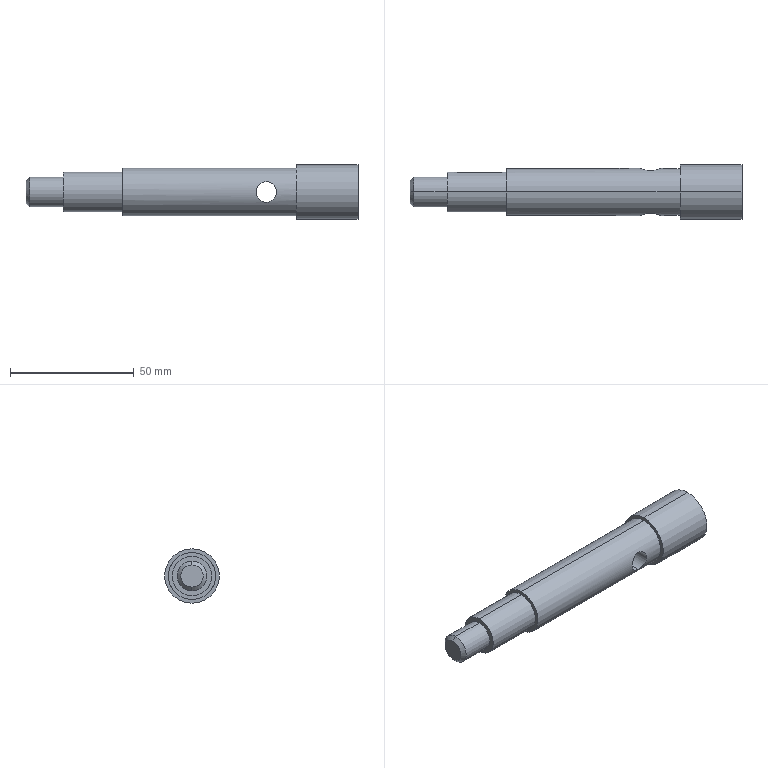Part | SolidWorks | features Cut 2, Chamfer 1, RevCut 1, Revolution 1 | 1 solid | 25 faces | box 134 x 22 x 22 mm | volume 34206 mm3 | cylinder 15 | plane 8 | cone 2 | commonest cylinder face diameters 2.8 x4 8.3 x2 12 x2 16 x2 19 x2 22 x2
STEP:
#1=CARTESIAN_POINT('',(-52.374,0.,4.5));
#2=VERTEX_POINT('',#1);
#3=CARTESIAN_POINT('',(-52.374,0.,-4.5));
#4=VERTEX_POINT('',#3);
#5=CARTESIAN_POINT('',(-52.374,0.,0.));
#6=DIRECTION('',(-1.,0.,0.));
#7=DIRECTION('',(0.,0.,-1.));
#8=AXIS2_PLACEMENT_3D('',#5,#6,#7);
#9=CIRCLE('',#8,4.5);
#10=EDGE_CURVE('',#2,#4,#9,.T.);
#11=ORIENTED_EDGE('',*,*,#10,.F.);
#12=CARTESIAN_POINT('',(-50.874,0.,6.));
#13=VERTEX_POINT('',#12);
#14=CARTESIAN_POINT('',(-52.374,0.,4.5));
#15=DIRECTION('',(0.7071,0.,0.7071));
#16=VECTOR('',#15,1000.);
#17=LINE('',#14,#16);
#18=EDGE_CURVE('',#2,#13,#17,.T.);
#19=ORIENTED_EDGE('',*,*,#18,.T.);
#20=CARTESIAN_POINT('',(-50.874,0.,-6.));
#21=VERTEX_POINT('',#20);
#22=CARTESIAN_POINT('',(-50.874,0.,0.));
#23=DIRECTION('',(1.,0.,0.));
#24=DIRECTION('',(0.,0.,-1.));
#25=AXIS2_PLACEMENT_3D('',#22,#23,#24);
#26=CIRCLE('',#25,6.);
#27=EDGE_CURVE('',#21,#13,#26,.T.);
#28=ORIENTED_EDGE('',*,*,#27,.F.);
#29=CARTESIAN_POINT('',(-52.374,0.,-4.5));
#30=DIRECTION('',(0.7071,0.,-0.7071));
#31=VECTOR('',#30,1000.);
#32=LINE('',#29,#31);
#33=EDGE_CURVE('',#4,#21,#32,.T.);
#34=ORIENTED_EDGE('',*,*,#33,.F.);
#35=EDGE_LOOP('',(#11,#19,#28,#34));
#36=FACE_OUTER_BOUND('',#35,.T.);
#37=CARTESIAN_POINT('',(-52.374,0.,0.));
#38=DIRECTION('',(1.,0.,0.));
#39=DIRECTION('',(0.,0.,-1.));
#40=AXIS2_PLACEMENT_3D('',#37,#38,#39);
#41=CONICAL_SURFACE('',#40,4.5,0.7854);
#42=ADVANCED_FACE('',(#36),#41,.T.);
#43=CARTESIAN_POINT('',(37.626,0.,1.4));
#44=VERTEX_POINT('',#43);
#45=CARTESIAN_POINT('',(37.626,0.,-1.4));
#46=VERTEX_POINT('',#45);
#47=CARTESIAN_POINT('',(37.626,0.,0.));
#48=DIRECTION('',(1.,0.,0.));
#49=DIRECTION('',(0.,0.,-1.));
#50=AXIS2_PLACEMENT_3D('',#47,#48,#49);
#51=CIRCLE('',#50,1.4);
#52=EDGE_CURVE('',#44,#46,#51,.T.);
#53=ORIENTED_EDGE('',*,*,#52,.F.);
#54=CARTESIAN_POINT('',(40.72,0.,1.4));
#55=VERTEX_POINT('',#54);
#56=CARTESIAN_POINT('',(37.626,0.,1.4));
#57=DIRECTION('',(1.,0.,0.));
#58=VECTOR('',#57,1000.);
#59=LINE('',#56,#58);
#60=EDGE_CURVE('',#44,#55,#59,.T.);
#61=ORIENTED_EDGE('',*,*,#60,.T.);
#62=CARTESIAN_POINT('',(40.72,0.,-1.4));
#63=VERTEX_POINT('',#62);
#64=CARTESIAN_POINT('',(40.72,0.,1.4));
#65=CARTESIAN_POINT('',(40.72,-0.1836,1.4));
#66=CARTESIAN_POINT('',(40.706,-0.369,1.363));
#67=CARTESIAN_POINT('',(40.671,-0.6223,1.257));
#68=CARTESIAN_POINT('',(40.657,-0.7041,1.213));
#69=CARTESIAN_POINT('',(40.628,-0.8552,1.112));
#70=CARTESIAN_POINT('',(40.612,-0.9252,1.055));
#71=CARTESIAN_POINT('',(40.564,-1.119,0.8607));
#72=CARTESIAN_POINT('',(40.534,-1.222,0.708));
#73=CARTESIAN_POINT('',(40.5,-1.328,0.4527));
#74=CARTESIAN_POINT('',(40.491,-1.355,0.3652));
#75=CARTESIAN_POINT('',(40.48,-1.391,0.1854));
#76=CARTESIAN_POINT('',(40.476,-1.4,0.092));
#77=CARTESIAN_POINT('',(40.476,-1.4,-0.1847));
#78=CARTESIAN_POINT('',(40.489,-1.363,-0.3697));
#79=CARTESIAN_POINT('',(40.533,-1.222,-0.7069));
#80=CARTESIAN_POINT('',(40.565,-1.118,-0.8618));
#81=CARTESIAN_POINT('',(40.612,-0.9256,-1.054));
#82=CARTESIAN_POINT('',(40.628,-0.8542,-1.113));
#83=CARTESIAN_POINT('',(40.658,-0.703,-1.214));
#84=CARTESIAN_POINT('',(40.671,-0.623,-1.257));
#85=CARTESIAN_POINT('',(40.694,-0.4537,-1.328));
#86=CARTESIAN_POINT('',(40.704,-0.3645,-1.355));
#87=CARTESIAN_POINT('',(40.716,-0.1848,-1.391));
#88=CARTESIAN_POINT('',(40.72,-0.09322,-1.4));
#89=CARTESIAN_POINT('',(40.72,0.,-1.4));
#90=B_SPLINE_CURVE_WITH_KNOTS('',3,(#64,#65,#66,#67,#68,#69,#70,#71,#72,#73,#74,#75,#76,#77,#78,#79,#80,#81,#82,#83,#84,#85,#86,#87,#88,#89),.UNSPECIFIED.,.F.,.F.,(4,2,2,2,2,2,2,2,2,2,2,2,4),(0.00441,0.004961,0.005236,0.005512,0.006063,0.006338,0.006614,0.007165,0.007716,0.007991,0.008267,0.008542,0.008818),.UNSPECIFIED.);
#91=EDGE_CURVE('',#55,#63,#90,.T.);
#92=ORIENTED_EDGE('',*,*,#91,.T.);
#93=CARTESIAN_POINT('',(37.626,0.,-1.4));
#94=DIRECTION('',(1.,0.,0.));
#95=VECTOR('',#94,1000.);
#96=LINE('',#93,#95);
#97=EDGE_CURVE('',#46,#63,#96,.T.);
#98=ORIENTED_EDGE('',*,*,#97,.F.);
#99=EDGE_LOOP('',(#53,#61,#92,#98));
#100=FACE_OUTER_BOUND('',#99,.T.);
#101=CARTESIAN_POINT('',(37.626,0.,0.));
#102=DIRECTION('',(1.,0.,0.));
#103=DIRECTION('',(0.,0.,-1.));
#104=AXIS2_PLACEMENT_3D('',#101,#102,#103);
#105=CYLINDRICAL_SURFACE('',#104,1.4);
#106=ADVANCED_FACE('',(#100),#105,.F.);
#107=CARTESIAN_POINT('',(40.72,0.,-1.4));
#108=CARTESIAN_POINT('',(40.72,0.09325,-1.4));
#109=CARTESIAN_POINT('',(40.716,0.1848,-1.391));
#110=CARTESIAN_POINT('',(40.704,0.3646,-1.355));
#111=CARTESIAN_POINT('',(40.694,0.4539,-1.328));
#112=CARTESIAN_POINT('',(40.66,0.7077,-1.222));
#113=CARTESIAN_POINT('',(40.628,0.862,-1.118));
#114=CARTESIAN_POINT('',(40.565,1.118,-0.8616));
#115=CARTESIAN_POINT('',(40.533,1.222,-0.7065));
#116=CARTESIAN_POINT('',(40.489,1.362,-0.37));
#117=CARTESIAN_POINT('',(40.476,1.4,-0.1849));
#118=CARTESIAN_POINT('',(40.476,1.4,0.09146));
#119=CARTESIAN_POINT('',(40.479,1.391,0.185));
#120=CARTESIAN_POINT('',(40.491,1.355,0.3652));
#121=CARTESIAN_POINT('',(40.5,1.328,0.4528));
#122=CARTESIAN_POINT('',(40.534,1.222,0.7085));
#123=CARTESIAN_POINT('',(40.565,1.118,0.8619));
#124=CARTESIAN_POINT('',(40.612,0.9248,1.055));
#125=CARTESIAN_POINT('',(40.628,0.8548,1.112));
#126=CARTESIAN_POINT('',(40.657,0.7036,1.214));
#127=CARTESIAN_POINT('',(40.671,0.6218,1.258));
#128=CARTESIAN_POINT('',(40.706,0.369,1.363));
#129=CARTESIAN_POINT('',(40.72,0.1837,1.4));
#130=CARTESIAN_POINT('',(40.72,0.,1.4));
#131=B_SPLINE_CURVE_WITH_KNOTS('',3,(#107,#108,#109,#110,#111,#112,#113,#114,#115,#116,#117,#118,#119,#120,#121,#122,#123,#124,#125,#126,#127,#128,#129,#130),.UNSPECIFIED.,.F.,.F.,(4,2,2,2,2,2,2,2,2,2,2,4),(0.,0.0002756,0.0005512,0.001102,0.001654,0.002205,0.00248,0.002756,0.003307,0.003583,0.003858,0.00441),.UNSPECIFIED.);
#132=EDGE_CURVE('',#63,#55,#131,.T.);
#133=ORIENTED_EDGE('',*,*,#132,.F.);
#134=ORIENTED_EDGE('',*,*,#91,.F.);
#135=EDGE_LOOP('',(#133,#134));
#136=FACE_BOUND('',#135,.T.);
#137=CARTESIAN_POINT('',(44.626,-8.546,-4.15));
#138=VERTEX_POINT('',#137);
#139=CARTESIAN_POINT('',(44.626,-8.546,4.15));
#140=VERTEX_POINT('',#139);
#141=CARTESIAN_POINT('',(44.626,-8.546,-4.15));
#142=CARTESIAN_POINT('',(44.353,-8.546,-4.15));
#143=CARTESIAN_POINT('',(44.075,-8.559,-4.122));
#144=CARTESIAN_POINT('',(43.538,-8.611,-4.014));
#145=CARTESIAN_POINT('',(43.278,-8.648,-3.934));
#146=CARTESIAN_POINT('',(42.776,-8.74,-3.724));
#147=CARTESIAN_POINT('',(42.536,-8.795,-3.595));
#148=CARTESIAN_POINT('',(42.091,-8.911,-3.296));
#149=CARTESIAN_POINT('',(41.881,-8.974,-3.124));
#150=CARTESIAN_POINT('',(41.501,-9.097,-2.744));
#151=CARTESIAN_POINT('',(41.331,-9.158,-2.537));
#152=CARTESIAN_POINT('',(41.032,-9.27,-2.092));
#153=CARTESIAN_POINT('',(40.901,-9.322,-1.849));
#154=CARTESIAN_POINT('',(40.693,-9.407,-1.349));
#155=CARTESIAN_POINT('',(40.613,-9.441,-1.09));
#156=CARTESIAN_POINT('',(40.504,-9.488,-0.5531));
#157=CARTESIAN_POINT('',(40.476,-9.5,-0.275));
#158=CARTESIAN_POINT('',(40.476,-9.5,0.2725));
#159=CARTESIAN_POINT('',(40.503,-9.488,0.5464));
#160=CARTESIAN_POINT('',(40.612,-9.441,1.088));
#161=CARTESIAN_POINT('',(40.692,-9.407,1.349));
#162=CARTESIAN_POINT('',(40.901,-9.322,1.849));
#163=CARTESIAN_POINT('',(41.032,-9.27,2.092));
#164=CARTESIAN_POINT('',(41.332,-9.158,2.538));
#165=CARTESIAN_POINT('',(41.502,-9.097,2.745));
#166=CARTESIAN_POINT('',(42.074,-8.911,3.316));
#167=CARTESIAN_POINT('',(42.523,-8.787,3.619));
#168=CARTESIAN_POINT('',(43.278,-8.648,3.934));
#169=CARTESIAN_POINT('',(43.538,-8.611,4.014));
#170=CARTESIAN_POINT('',(44.071,-8.56,4.122));
#171=CARTESIAN_POINT('',(44.349,-8.546,4.15));
#172=CARTESIAN_POINT('',(44.626,-8.546,4.15));
#173=B_SPLINE_CURVE_WITH_KNOTS('',3,(#141,#142,#143,#144,#145,#146,#147,#148,#149,#150,#151,#152,#153,#154,#155,#156,#157,#158,#159,#160,#161,#162,#163,#164,#165,#166,#167,#168,#169,#170,#171,#172),.UNSPECIFIED.,.F.,.F.,(4,2,2,2,2,2,2,2,2,2,2,2,2,2,2,4),(0.01314,0.01396,0.01478,0.0156,0.01642,0.01724,0.01806,0.01889,0.01971,0.02053,0.02135,0.02217,0.02299,0.02463,0.02545,0.02627),.UNSPECIFIED.);
#174=EDGE_CURVE('',#138,#140,#173,.T.);
#175=ORIENTED_EDGE('',*,*,#174,.F.);
#176=CARTESIAN_POINT('',(44.626,8.546,-4.15));
#177=VERTEX_POINT('',#176);
#178=CARTESIAN_POINT('',(44.626,-11.,-4.15));
#179=DIRECTION('',(0.,1.,0.));
#180=VECTOR('',#179,1000.);
#181=LINE('',#178,#180);
#182=EDGE_CURVE('',#138,#177,#181,.T.);
#183=ORIENTED_EDGE('',*,*,#182,.T.);
#184=CARTESIAN_POINT('',(44.626,8.546,4.15));
#185=VERTEX_POINT('',#184);
#186=CARTESIAN_POINT('',(44.626,8.546,4.15));
#187=CARTESIAN_POINT('',(44.348,8.546,4.15));
#188=CARTESIAN_POINT('',(44.076,8.559,4.122));
#189=CARTESIAN_POINT('',(43.541,8.61,4.015));
#190=CARTESIAN_POINT('',(43.276,8.648,3.933));
#191=CARTESIAN_POINT('',(42.775,8.74,3.724));
#192=CARTESIAN_POINT('',(42.538,8.794,3.597));
#193=CARTESIAN_POINT('',(42.09,8.911,3.296));
#194=CARTESIAN_POINT('',(41.881,8.974,3.124));
#195=CARTESIAN_POINT('',(41.503,9.097,2.746));
#196=CARTESIAN_POINT('',(41.331,9.158,2.538));
#197=CARTESIAN_POINT('',(41.029,9.271,2.088));
#198=CARTESIAN_POINT('',(40.902,9.321,1.851));
#199=CARTESIAN_POINT('',(40.693,9.407,1.352));
#200=CARTESIAN_POINT('',(40.612,9.441,1.087));
#201=CARTESIAN_POINT('',(40.504,9.488,0.5491));
#202=CARTESIAN_POINT('',(40.477,9.5,0.2772));
#203=CARTESIAN_POINT('',(40.476,9.5,-0.2726));
#204=CARTESIAN_POINT('',(40.504,9.488,-0.5512));
#205=CARTESIAN_POINT('',(40.612,9.441,-1.087));
#206=CARTESIAN_POINT('',(40.692,9.407,-1.349));
#207=CARTESIAN_POINT('',(40.904,9.321,-1.854));
#208=CARTESIAN_POINT('',(41.032,9.27,-2.092));
#209=CARTESIAN_POINT('',(41.332,9.158,-2.538));
#210=CARTESIAN_POINT('',(41.506,9.096,-2.749));
#211=CARTESIAN_POINT('',(41.885,8.973,-3.127));
#212=CARTESIAN_POINT('',(42.091,8.911,-3.297));
#213=CARTESIAN_POINT('',(42.539,8.794,-3.597));
#214=CARTESIAN_POINT('',(42.78,8.739,-3.726));
#215=CARTESIAN_POINT('',(43.278,8.648,-3.934));
#216=CARTESIAN_POINT('',(43.537,8.611,-4.014));
#217=CARTESIAN_POINT('',(44.08,8.559,-4.123));
#218=CARTESIAN_POINT('',(44.353,8.546,-4.15));
#219=CARTESIAN_POINT('',(44.626,8.546,-4.15));
#220=B_SPLINE_CURVE_WITH_KNOTS('',3,(#186,#187,#188,#189,#190,#191,#192,#193,#194,#195,#196,#197,#198,#199,#200,#201,#202,#203,#204,#205,#206,#207,#208,#209,#210,#211,#212,#213,#214,#215,#216,#217,#218,#219),.UNSPECIFIED.,.F.,.F.,(4,2,2,2,2,2,2,2,2,2,2,2,2,2,2,2,4),(0.,0.0008214,0.001643,0.002464,0.003285,0.004107,0.004928,0.00575,0.006571,0.007392,0.008214,0.009035,0.009856,0.01068,0.0115,0.01232,0.01314),.UNSPECIFIED.);
#221=EDGE_CURVE('',#185,#177,#220,.T.);
#222=ORIENTED_EDGE('',*,*,#221,.F.);
#223=CARTESIAN_POINT('',(44.626,-11.,4.15));
#224=DIRECTION('',(0.,1.,0.));
#225=VECTOR('',#224,1000.);
#226=LINE('',#223,#225);
#227=EDGE_CURVE('',#140,#185,#226,.T.);
#228=ORIENTED_EDGE('',*,*,#227,.F.);
#229=EDGE_LOOP('',(#175,#183,#222,#228));
#230=FACE_OUTER_BOUND('',#229,.T.);
#231=CARTESIAN_POINT('',(44.626,-11.,0.));
#232=DIRECTION('',(0.,1.,0.));
#233=DIRECTION('',(0.,0.,1.));
#234=AXIS2_PLACEMENT_3D('',#231,#232,#233);
#235=CYLINDRICAL_SURFACE('',#234,4.15);
#236=ADVANCED_FACE('',(#136,#230),#235,.F.);
#237=CARTESIAN_POINT('',(48.533,0.,-1.4));
#238=VERTEX_POINT('',#237);
#239=CARTESIAN_POINT('',(48.533,0.,1.4));
#240=VERTEX_POINT('',#239);
#241=CARTESIAN_POINT('',(48.533,0.,-1.4));
#242=CARTESIAN_POINT('',(48.533,-0.09325,-1.4));
#243=CARTESIAN_POINT('',(48.536,-0.1848,-1.391));
#244=CARTESIAN_POINT('',(48.549,-0.3646,-1.355));
#245=CARTESIAN_POINT('',(48.558,-0.4539,-1.328));
#246=CARTESIAN_POINT('',(48.593,-0.7077,-1.222));
#247=CARTESIAN_POINT('',(48.625,-0.862,-1.118));
#248=CARTESIAN_POINT('',(48.688,-1.118,-0.8616));
#249=CARTESIAN_POINT('',(48.719,-1.222,-0.7065));
#250=CARTESIAN_POINT('',(48.763,-1.362,-0.37));
#251=CARTESIAN_POINT('',(48.776,-1.4,-0.1849));
#252=CARTESIAN_POINT('',(48.776,-1.4,0.09146));
#253=CARTESIAN_POINT('',(48.773,-1.391,0.185));
#254=CARTESIAN_POINT('',(48.761,-1.355,0.3652));
#255=CARTESIAN_POINT('',(48.752,-1.328,0.4528));
#256=CARTESIAN_POINT('',(48.719,-1.222,0.7085));
#257=CARTESIAN_POINT('',(48.688,-1.118,0.8619));
#258=CARTESIAN_POINT('',(48.641,-0.9248,1.055));
#259=CARTESIAN_POINT('',(48.625,-0.8548,1.112));
#260=CARTESIAN_POINT('',(48.595,-0.7036,1.214));
#261=CARTESIAN_POINT('',(48.581,-0.6218,1.258));
#262=CARTESIAN_POINT('',(48.547,-0.369,1.363));
#263=CARTESIAN_POINT('',(48.533,-0.1837,1.4));
#264=CARTESIAN_POINT('',(48.533,0.,1.4));
#265=B_SPLINE_CURVE_WITH_KNOTS('',3,(#241,#242,#243,#244,#245,#246,#247,#248,#249,#250,#251,#252,#253,#254,#255,#256,#257,#258,#259,#260,#261,#262,#263,#264),.UNSPECIFIED.,.F.,.F.,(4,2,2,2,2,2,2,2,2,2,2,4),(0.,0.0002756,0.0005512,0.001102,0.001654,0.002205,0.00248,0.002756,0.003307,0.003583,0.003858,0.00441),.UNSPECIFIED.);
#266=EDGE_CURVE('',#238,#240,#265,.T.);
#267=ORIENTED_EDGE('',*,*,#266,.T.);
#268=CARTESIAN_POINT('',(81.626,0.,1.4));
#269=VERTEX_POINT('',#268);
#270=CARTESIAN_POINT('',(37.626,0.,1.4));
#271=DIRECTION('',(1.,0.,0.));
#272=VECTOR('',#271,1000.);
#273=LINE('',#270,#272);
#274=EDGE_CURVE('',#240,#269,#273,.T.);
#275=ORIENTED_EDGE('',*,*,#274,.T.);
#276=CARTESIAN_POINT('',(81.626,0.,-1.4));
#277=VERTEX_POINT('',#276);
#278=CARTESIAN_POINT('',(81.626,0.,0.));
#279=DIRECTION('',(1.,0.,0.));
#280=DIRECTION('',(0.,0.,-1.));
#281=AXIS2_PLACEMENT_3D('',#278,#279,#280);
#282=CIRCLE('',#281,1.4);
#283=EDGE_CURVE('',#269,#277,#282,.T.);
#284=ORIENTED_EDGE('',*,*,#283,.T.);
#285=CARTESIAN_POINT('',(37.626,0.,-1.4));
#286=DIRECTION('',(1.,0.,0.));
#287=VECTOR('',#286,1000.);
#288=LINE('',#285,#287);
#289=EDGE_CURVE('',#238,#277,#288,.T.);
#290=ORIENTED_EDGE('',*,*,#289,.F.);
#291=EDGE_LOOP('',(#267,#275,#284,#290));
#292=FACE_OUTER_BOUND('',#291,.T.);
#293=CARTESIAN_POINT('',(37.626,0.,0.));
#294=DIRECTION('',(1.,0.,0.));
#295=DIRECTION('',(0.,0.,-1.));
#296=AXIS2_PLACEMENT_3D('',#293,#294,#295);
#297=CYLINDRICAL_SURFACE('',#296,1.4);
#298=ADVANCED_FACE('',(#292),#297,.F.);
#299=CARTESIAN_POINT('',(-37.374,0.,6.));
#300=VERTEX_POINT('',#299);
#301=CARTESIAN_POINT('',(-37.374,0.,-6.));
#302=VERTEX_POINT('',#301);
#303=CARTESIAN_POINT('',(-37.374,0.,0.));
#304=DIRECTION('',(-1.,0.,0.));
#305=DIRECTION('',(0.,0.,1.));
#306=AXIS2_PLACEMENT_3D('',#303,#304,#305);
#307=CIRCLE('',#306,6.);
#308=EDGE_CURVE('',#300,#302,#307,.T.);
#309=ORIENTED_EDGE('',*,*,#308,.T.);
#310=CARTESIAN_POINT('',(-52.374,0.,-6.));
#311=DIRECTION('',(-1.,0.,0.));
#312=VECTOR('',#311,1000.);
#313=LINE('',#310,#312);
#314=EDGE_CURVE('',#302,#21,#313,.T.);
#315=ORIENTED_EDGE('',*,*,#314,.T.);
#316=ORIENTED_EDGE('',*,*,#27,.T.);
#317=CARTESIAN_POINT('',(-52.374,0.,6.));
#318=DIRECTION('',(-1.,0.,0.));
#319=VECTOR('',#318,1000.);
#320=LINE('',#317,#319);
#321=EDGE_CURVE('',#300,#13,#320,.T.);
#322=ORIENTED_EDGE('',*,*,#321,.F.);
#323=EDGE_LOOP('',(#309,#315,#316,#322));
#324=FACE_OUTER_BOUND('',#323,.T.);
#325=CARTESIAN_POINT('',(-52.374,0.,0.));
#326=DIRECTION('',(-1.,0.,0.));
#327=DIRECTION('',(0.,0.,1.));
#328=AXIS2_PLACEMENT_3D('',#325,#326,#327);
#329=CYLINDRICAL_SURFACE('',#328,6.);
#330=ADVANCED_FACE('',(#324),#329,.T.);
#331=CARTESIAN_POINT('',(-33.372,7.838,-1.6));
#332=VERTEX_POINT('',#331);
#333=CARTESIAN_POINT('',(-15.375,7.838,-1.6));
#334=VERTEX_POINT('',#333);
#335=CARTESIAN_POINT('',(-52.374,7.838,-1.6));
#336=DIRECTION('',(1.,0.,0.));
#337=VECTOR('',#336,1000.);
#338=LINE('',#335,#337);
#339=EDGE_CURVE('',#332,#334,#338,.T.);
#340=ORIENTED_EDGE('',*,*,#339,.T.);
#341=CARTESIAN_POINT('',(-15.374,8.,0.));
#342=VERTEX_POINT('',#341);
#343=CARTESIAN_POINT('',(-15.375,7.838,-1.6));
#344=CARTESIAN_POINT('',(-15.373,7.947,-1.068));
#345=CARTESIAN_POINT('',(-15.374,8.,-0.5351));
#346=CARTESIAN_POINT('',(-15.374,8.,0.));
#347=B_SPLINE_CURVE_WITH_KNOTS('',3,(#343,#344,#345,#346),.UNSPECIFIED.,.F.,.F.,(4,4),(0.,0.001604),.UNSPECIFIED.);
#348=EDGE_CURVE('',#334,#342,#347,.T.);
#349=ORIENTED_EDGE('',*,*,#348,.T.);
#350=CARTESIAN_POINT('',(-15.375,7.838,1.6));
#351=VERTEX_POINT('',#350);
#352=CARTESIAN_POINT('',(-15.374,8.,0.));
#353=CARTESIAN_POINT('',(-15.374,8.,0.5327));
#354=CARTESIAN_POINT('',(-15.373,7.946,1.071));
#355=CARTESIAN_POINT('',(-15.375,7.838,1.6));
#356=B_SPLINE_CURVE_WITH_KNOTS('',3,(#352,#353,#354,#355),.UNSPECIFIED.,.F.,.F.,(4,4),(0.001604,0.003202),.UNSPECIFIED.);
#357=EDGE_CURVE('',#342,#351,#356,.T.);
#358=ORIENTED_EDGE('',*,*,#357,.T.);
#359=CARTESIAN_POINT('',(-33.372,7.838,1.6));
#360=VERTEX_POINT('',#359);
#361=CARTESIAN_POINT('',(-52.374,7.838,1.6));
#362=DIRECTION('',(-1.,0.,0.));
#363=VECTOR('',#362,1000.);
#364=LINE('',#361,#363);
#365=EDGE_CURVE('',#351,#360,#364,.T.);
#366=ORIENTED_EDGE('',*,*,#365,.T.);
#367=CARTESIAN_POINT('',(-33.374,8.,0.));
#368=VERTEX_POINT('',#367);
#369=CARTESIAN_POINT('',(-33.372,7.838,1.6));
#370=CARTESIAN_POINT('',(-33.374,7.947,1.068));
#371=CARTESIAN_POINT('',(-33.374,8.,0.5351));
#372=CARTESIAN_POINT('',(-33.374,8.,0.));
#373=B_SPLINE_CURVE_WITH_KNOTS('',3,(#369,#370,#371,#372),.UNSPECIFIED.,.F.,.F.,(4,4),(0.,0.001604),.UNSPECIFIED.);
#374=EDGE_CURVE('',#360,#368,#373,.T.);
#375=ORIENTED_EDGE('',*,*,#374,.T.);
#376=CARTESIAN_POINT('',(-33.374,8.,0.));
#377=CARTESIAN_POINT('',(-33.374,8.,-0.5327));
#378=CARTESIAN_POINT('',(-33.374,7.946,-1.071));
#379=CARTESIAN_POINT('',(-33.372,7.838,-1.6));
#380=B_SPLINE_CURVE_WITH_KNOTS('',3,(#376,#377,#378,#379),.UNSPECIFIED.,.F.,.F.,(4,4),(0.001604,0.003202),.UNSPECIFIED.);
#381=EDGE_CURVE('',#368,#332,#380,.T.);
#382=ORIENTED_EDGE('',*,*,#381,.T.);
#383=EDGE_LOOP('',(#340,#349,#358,#366,#375,#382));
#384=FACE_BOUND('',#383,.T.);
#385=CARTESIAN_POINT('',(-13.374,0.,8.));
#386=VERTEX_POINT('',#385);
#387=CARTESIAN_POINT('',(-13.374,0.,-8.));
#388=VERTEX_POINT('',#387);
#389=CARTESIAN_POINT('',(-13.374,0.,0.));
#390=DIRECTION('',(-1.,0.,0.));
#391=DIRECTION('',(0.,0.,1.));
#392=AXIS2_PLACEMENT_3D('',#389,#390,#391);
#393=CIRCLE('',#392,8.);
#394=EDGE_CURVE('',#386,#388,#393,.T.);
#395=ORIENTED_EDGE('',*,*,#394,.T.);
#396=CARTESIAN_POINT('',(-37.374,0.,-8.));
#397=VERTEX_POINT('',#396);
#398=CARTESIAN_POINT('',(-52.374,0.,-8.));
#399=DIRECTION('',(-1.,0.,0.));
#400=VECTOR('',#399,1000.);
#401=LINE('',#398,#400);
#402=EDGE_CURVE('',#388,#397,#401,.T.);
#403=ORIENTED_EDGE('',*,*,#402,.T.);
#404=CARTESIAN_POINT('',(-37.374,0.,8.));
#405=VERTEX_POINT('',#404);
#406=CARTESIAN_POINT('',(-37.374,0.,0.));
#407=DIRECTION('',(-1.,0.,0.));
#408=DIRECTION('',(0.,0.,1.));
#409=AXIS2_PLACEMENT_3D('',#406,#407,#408);
#410=CIRCLE('',#409,8.);
#411=EDGE_CURVE('',#405,#397,#410,.T.);
#412=ORIENTED_EDGE('',*,*,#411,.F.);
#413=CARTESIAN_POINT('',(-52.374,0.,8.));
#414=DIRECTION('',(-1.,0.,0.));
#415=VECTOR('',#414,1000.);
#416=LINE('',#413,#415);
#417=EDGE_CURVE('',#386,#405,#416,.T.);
#418=ORIENTED_EDGE('',*,*,#417,.F.);
#419=EDGE_LOOP('',(#395,#403,#412,#418));
#420=FACE_OUTER_BOUND('',#419,.T.);
#421=CARTESIAN_POINT('',(-52.374,0.,0.));
#422=DIRECTION('',(-1.,0.,0.));
#423=DIRECTION('',(0.,0.,1.));
#424=AXIS2_PLACEMENT_3D('',#421,#422,#423);
#425=CYLINDRICAL_SURFACE('',#424,8.);
#426=ADVANCED_FACE('',(#384,#420),#425,.T.);
#427=ORIENTED_EDGE('',*,*,#221,.T.);
#428=CARTESIAN_POINT('',(44.626,8.546,-4.15));
#429=CARTESIAN_POINT('',(44.9,8.546,-4.15));
#430=CARTESIAN_POINT('',(45.178,8.559,-4.122));
#431=CARTESIAN_POINT('',(45.715,8.611,-4.014));
#432=CARTESIAN_POINT('',(45.975,8.648,-3.934));
#433=CARTESIAN_POINT('',(46.477,8.74,-3.724));
#434=CARTESIAN_POINT('',(46.717,8.795,-3.595));
#435=CARTESIAN_POINT('',(47.162,8.911,-3.296));
#436=CARTESIAN_POINT('',(47.371,8.974,-3.124));
#437=CARTESIAN_POINT('',(47.752,9.097,-2.744));
#438=CARTESIAN_POINT('',(47.921,9.158,-2.537));
#439=CARTESIAN_POINT('',(48.221,9.27,-2.092));
#440=CARTESIAN_POINT('',(48.351,9.322,-1.849));
#441=CARTESIAN_POINT('',(48.56,9.407,-1.349));
#442=CARTESIAN_POINT('',(48.64,9.441,-1.09));
#443=CARTESIAN_POINT('',(48.748,9.488,-0.5531));
#444=CARTESIAN_POINT('',(48.776,9.5,-0.275));
#445=CARTESIAN_POINT('',(48.776,9.5,0.2725));
#446=CARTESIAN_POINT('',(48.749,9.488,0.5464));
#447=CARTESIAN_POINT('',(48.641,9.441,1.088));
#448=CARTESIAN_POINT('',(48.56,9.407,1.349));
#449=CARTESIAN_POINT('',(48.351,9.322,1.849));
#450=CARTESIAN_POINT('',(48.221,9.27,2.092));
#451=CARTESIAN_POINT('',(47.921,9.158,2.538));
#452=CARTESIAN_POINT('',(47.751,9.097,2.745));
#453=CARTESIAN_POINT('',(47.179,8.911,3.316));
#454=CARTESIAN_POINT('',(46.73,8.787,3.619));
#455=CARTESIAN_POINT('',(45.974,8.648,3.934));
#456=CARTESIAN_POINT('',(45.715,8.611,4.014));
#457=CARTESIAN_POINT('',(45.181,8.56,4.122));
#458=CARTESIAN_POINT('',(44.904,8.546,4.15));
#459=CARTESIAN_POINT('',(44.626,8.546,4.15));
#460=B_SPLINE_CURVE_WITH_KNOTS('',3,(#428,#429,#430,#431,#432,#433,#434,#435,#436,#437,#438,#439,#440,#441,#442,#443,#444,#445,#446,#447,#448,#449,#450,#451,#452,#453,#454,#455,#456,#457,#458,#459),.UNSPECIFIED.,.F.,.F.,(4,2,2,2,2,2,2,2,2,2,2,2,2,2,2,4),(0.01314,0.01396,0.01478,0.0156,0.01642,0.01724,0.01806,0.01889,0.01971,0.02053,0.02135,0.02217,0.02299,0.02463,0.02545,0.02627),.UNSPECIFIED.);
#461=EDGE_CURVE('',#177,#185,#460,.T.);
#462=ORIENTED_EDGE('',*,*,#461,.T.);
#463=EDGE_LOOP('',(#427,#462));
#464=FACE_BOUND('',#463,.T.);
#465=CARTESIAN_POINT('',(56.626,0.,9.5));
#466=VERTEX_POINT('',#465);
#467=CARTESIAN_POINT('',(56.626,0.,-9.5));
#468=VERTEX_POINT('',#467);
#469=CARTESIAN_POINT('',(56.626,0.,0.));
#470=DIRECTION('',(-1.,0.,0.));
#471=DIRECTION('',(0.,0.,1.));
#472=AXIS2_PLACEMENT_3D('',#469,#470,#471);
#473=CIRCLE('',#472,9.5);
#474=EDGE_CURVE('',#466,#468,#473,.T.);
#475=ORIENTED_EDGE('',*,*,#474,.T.);
#476=CARTESIAN_POINT('',(-13.374,0.,-9.5));
#477=VERTEX_POINT('',#476);
#478=CARTESIAN_POINT('',(-52.374,0.,-9.5));
#479=DIRECTION('',(-1.,0.,0.));
#480=VECTOR('',#479,1000.);
#481=LINE('',#478,#480);
#482=EDGE_CURVE('',#468,#477,#481,.T.);
#483=ORIENTED_EDGE('',*,*,#482,.T.);
#484=CARTESIAN_POINT('',(-13.374,0.,9.5));
#485=VERTEX_POINT('',#484);
#486=CARTESIAN_POINT('',(-13.374,0.,0.));
#487=DIRECTION('',(-1.,0.,0.));
#488=DIRECTION('',(0.,0.,1.));
#489=AXIS2_PLACEMENT_3D('',#486,#487,#488);
#490=CIRCLE('',#489,9.5);
#491=EDGE_CURVE('',#485,#477,#490,.T.);
#492=ORIENTED_EDGE('',*,*,#491,.F.);
#493=CARTESIAN_POINT('',(-52.374,0.,9.5));
#494=DIRECTION('',(-1.,0.,0.));
#495=VECTOR('',#494,1000.);
#496=LINE('',#493,#495);
#497=EDGE_CURVE('',#466,#485,#496,.T.);
#498=ORIENTED_EDGE('',*,*,#497,.F.);
#499=EDGE_LOOP('',(#475,#483,#492,#498));
#500=FACE_OUTER_BOUND('',#499,.T.);
#501=CARTESIAN_POINT('',(-52.374,0.,0.));
#502=DIRECTION('',(-1.,0.,0.));
#503=DIRECTION('',(0.,0.,1.));
#504=AXIS2_PLACEMENT_3D('',#501,#502,#503);
#505=CYLINDRICAL_SURFACE('',#504,9.5);
#506=ADVANCED_FACE('',(#464,#500),#505,.T.);
#507=CARTESIAN_POINT('',(81.626,0.,11.));
#508=VERTEX_POINT('',#507);
#509=CARTESIAN_POINT('',(81.626,0.,-11.));
#510=VERTEX_POINT('',#509);
#511=CARTESIAN_POINT('',(81.626,0.,0.));
#512=DIRECTION('',(-1.,0.,0.));
#513=DIRECTION('',(0.,0.,1.));
#514=AXIS2_PLACEMENT_3D('',#511,#512,#513);
#515=CIRCLE('',#514,11.);
#516=EDGE_CURVE('',#508,#510,#515,.T.);
#517=ORIENTED_EDGE('',*,*,#516,.T.);
#518=CARTESIAN_POINT('',(56.626,0.,-11.));
#519=VERTEX_POINT('',#518);
#520=CARTESIAN_POINT('',(-52.374,0.,-11.));
#521=DIRECTION('',(-1.,0.,0.));
#522=VECTOR('',#521,1000.);
#523=LINE('',#520,#522);
#524=EDGE_CURVE('',#510,#519,#523,.T.);
#525=ORIENTED_EDGE('',*,*,#524,.T.);
#526=CARTESIAN_POINT('',(56.626,0.,11.));
#527=VERTEX_POINT('',#526);
#528=CARTESIAN_POINT('',(56.626,0.,0.));
#529=DIRECTION('',(-1.,0.,0.));
#530=DIRECTION('',(0.,0.,1.));
#531=AXIS2_PLACEMENT_3D('',#528,#529,#530);
#532=CIRCLE('',#531,11.);
#533=EDGE_CURVE('',#527,#519,#532,.T.);
#534=ORIENTED_EDGE('',*,*,#533,.F.);
#535=CARTESIAN_POINT('',(-52.374,0.,11.));
#536=DIRECTION('',(-1.,0.,0.));
#537=VECTOR('',#536,1000.);
#538=LINE('',#535,#537);
#539=EDGE_CURVE('',#508,#527,#538,.T.);
#540=ORIENTED_EDGE('',*,*,#539,.F.);
#541=EDGE_LOOP('',(#517,#525,#534,#540));
#542=FACE_OUTER_BOUND('',#541,.T.);
#543=CARTESIAN_POINT('',(-52.374,0.,0.));
#544=DIRECTION('',(-1.,0.,0.));
#545=DIRECTION('',(0.,0.,1.));
#546=AXIS2_PLACEMENT_3D('',#543,#544,#545);
#547=CYLINDRICAL_SURFACE('',#546,11.);
#548=ADVANCED_FACE('',(#542),#547,.T.);
#549=CARTESIAN_POINT('',(81.626,0.,0.));
#550=DIRECTION('',(1.,0.,0.));
#551=DIRECTION('',(0.,0.,-1.));
#552=AXIS2_PLACEMENT_3D('',#549,#550,#551);
#553=CIRCLE('',#552,1.4);
#554=EDGE_CURVE('',#277,#269,#553,.T.);
#555=ORIENTED_EDGE('',*,*,#554,.F.);
#556=ORIENTED_EDGE('',*,*,#283,.F.);
#557=EDGE_LOOP('',(#555,#556));
#558=FACE_BOUND('',#557,.T.);
#559=ORIENTED_EDGE('',*,*,#516,.F.);
#560=CARTESIAN_POINT('',(81.626,0.,0.));
#561=DIRECTION('',(-1.,0.,0.));
#562=DIRECTION('',(0.,0.,1.));
#563=AXIS2_PLACEMENT_3D('',#560,#561,#562);
#564=CIRCLE('',#563,11.);
#565=EDGE_CURVE('',#510,#508,#564,.T.);
#566=ORIENTED_EDGE('',*,*,#565,.F.);
#567=EDGE_LOOP('',(#559,#566));
#568=FACE_OUTER_BOUND('',#567,.T.);
#569=CARTESIAN_POINT('',(81.626,0.,-11.));
#570=DIRECTION('',(-1.,0.,0.));
#571=DIRECTION('',(0.,0.,1.));
#572=AXIS2_PLACEMENT_3D('',#569,#570,#571);
#573=PLANE('',#572);
#574=ADVANCED_FACE('',(#558,#568),#573,.F.);
#575=ORIENTED_EDGE('',*,*,#524,.F.);
#576=ORIENTED_EDGE('',*,*,#565,.T.);
#577=ORIENTED_EDGE('',*,*,#539,.T.);
#578=CARTESIAN_POINT('',(56.626,0.,0.));
#579=DIRECTION('',(-1.,0.,0.));
#580=DIRECTION('',(0.,0.,1.));
#581=AXIS2_PLACEMENT_3D('',#578,#579,#580);
#582=CIRCLE('',#581,11.);
#583=EDGE_CURVE('',#519,#527,#582,.T.);
#584=ORIENTED_EDGE('',*,*,#583,.F.);
#585=EDGE_LOOP('',(#575,#576,#577,#584));
#586=FACE_OUTER_BOUND('',#585,.T.);
#587=CARTESIAN_POINT('',(-52.374,0.,0.));
#588=DIRECTION('',(-1.,0.,0.));
#589=DIRECTION('',(0.,0.,1.));
#590=AXIS2_PLACEMENT_3D('',#587,#588,#589);
#591=CYLINDRICAL_SURFACE('',#590,11.);
#592=ADVANCED_FACE('',(#586),#591,.T.);
#593=ORIENTED_EDGE('',*,*,#474,.F.);
#594=CARTESIAN_POINT('',(56.626,0.,0.));
#595=DIRECTION('',(-1.,0.,0.));
#596=DIRECTION('',(0.,0.,1.));
#597=AXIS2_PLACEMENT_3D('',#594,#595,#596);
#598=CIRCLE('',#597,9.5);
#599=EDGE_CURVE('',#468,#466,#598,.T.);
#600=ORIENTED_EDGE('',*,*,#599,.F.);
#601=EDGE_LOOP('',(#593,#600));
#602=FACE_BOUND('',#601,.T.);
#603=ORIENTED_EDGE('',*,*,#533,.T.);
#604=ORIENTED_EDGE('',*,*,#583,.T.);
#605=EDGE_LOOP('',(#603,#604));
#606=FACE_OUTER_BOUND('',#605,.T.);
#607=CARTESIAN_POINT('',(56.626,0.,-9.5));
#608=DIRECTION('',(1.,0.,0.));
#609=DIRECTION('',(0.,0.,-1.));
#610=AXIS2_PLACEMENT_3D('',#607,#608,#609);
#611=PLANE('',#610);
#612=ADVANCED_FACE('',(#602,#606),#611,.F.);
#613=ORIENTED_EDGE('',*,*,#482,.F.);
#614=ORIENTED_EDGE('',*,*,#599,.T.);
#615=ORIENTED_EDGE('',*,*,#497,.T.);
#616=CARTESIAN_POINT('',(-13.374,0.,0.));
#617=DIRECTION('',(-1.,0.,0.));
#618=DIRECTION('',(0.,0.,1.));
#619=AXIS2_PLACEMENT_3D('',#616,#617,#618);
#620=CIRCLE('',#619,9.5);
#621=EDGE_CURVE('',#477,#485,#620,.T.);
#622=ORIENTED_EDGE('',*,*,#621,.F.);
#623=EDGE_LOOP('',(#613,#614,#615,#622));
#624=FACE_OUTER_BOUND('',#623,.T.);
#625=CARTESIAN_POINT('',(44.626,-8.546,4.15));
#626=CARTESIAN_POINT('',(44.904,-8.546,4.15));
#627=CARTESIAN_POINT('',(45.177,-8.559,4.122));
#628=CARTESIAN_POINT('',(45.712,-8.61,4.015));
#629=CARTESIAN_POINT('',(45.977,-8.648,3.933));
#630=CARTESIAN_POINT('',(46.478,-8.74,3.724));
#631=CARTESIAN_POINT('',(46.715,-8.794,3.597));
#632=CARTESIAN_POINT('',(47.163,-8.911,3.296));
#633=CARTESIAN_POINT('',(47.372,-8.974,3.124));
#634=CARTESIAN_POINT('',(47.75,-9.097,2.746));
#635=CARTESIAN_POINT('',(47.921,-9.158,2.538));
#636=CARTESIAN_POINT('',(48.223,-9.271,2.088));
#637=CARTESIAN_POINT('',(48.351,-9.321,1.851));
#638=CARTESIAN_POINT('',(48.559,-9.407,1.352));
#639=CARTESIAN_POINT('',(48.641,-9.441,1.087));
#640=CARTESIAN_POINT('',(48.749,-9.488,0.5491));
#641=CARTESIAN_POINT('',(48.776,-9.5,0.2772));
#642=CARTESIAN_POINT('',(48.777,-9.5,-0.2726));
#643=CARTESIAN_POINT('',(48.749,-9.488,-0.5512));
#644=CARTESIAN_POINT('',(48.641,-9.441,-1.087));
#645=CARTESIAN_POINT('',(48.561,-9.407,-1.349));
#646=CARTESIAN_POINT('',(48.349,-9.321,-1.854));
#647=CARTESIAN_POINT('',(48.221,-9.27,-2.092));
#648=CARTESIAN_POINT('',(47.921,-9.158,-2.538));
#649=CARTESIAN_POINT('',(47.747,-9.096,-2.749));
#650=CARTESIAN_POINT('',(47.368,-8.973,-3.127));
#651=CARTESIAN_POINT('',(47.161,-8.911,-3.297));
#652=CARTESIAN_POINT('',(46.713,-8.794,-3.597));
#653=CARTESIAN_POINT('',(46.473,-8.739,-3.726));
#654=CARTESIAN_POINT('',(45.975,-8.648,-3.934));
#655=CARTESIAN_POINT('',(45.716,-8.611,-4.014));
#656=CARTESIAN_POINT('',(45.173,-8.559,-4.123));
#657=CARTESIAN_POINT('',(44.9,-8.546,-4.15));
#658=CARTESIAN_POINT('',(44.626,-8.546,-4.15));
#659=B_SPLINE_CURVE_WITH_KNOTS('',3,(#625,#626,#627,#628,#629,#630,#631,#632,#633,#634,#635,#636,#637,#638,#639,#640,#641,#642,#643,#644,#645,#646,#647,#648,#649,#650,#651,#652,#653,#654,#655,#656,#657,#658),.UNSPECIFIED.,.F.,.F.,(4,2,2,2,2,2,2,2,2,2,2,2,2,2,2,2,4),(0.,0.0008214,0.001643,0.002464,0.003285,0.004107,0.004928,0.00575,0.006571,0.007392,0.008214,0.009035,0.009856,0.01068,0.0115,0.01232,0.01314),.UNSPECIFIED.);
#660=EDGE_CURVE('',#140,#138,#659,.T.);
#661=ORIENTED_EDGE('',*,*,#660,.T.);
#662=ORIENTED_EDGE('',*,*,#174,.T.);
#663=EDGE_LOOP('',(#661,#662));
#664=FACE_BOUND('',#663,.T.);
#665=CARTESIAN_POINT('',(-52.374,0.,0.));
#666=DIRECTION('',(-1.,0.,0.));
#667=DIRECTION('',(0.,0.,1.));
#668=AXIS2_PLACEMENT_3D('',#665,#666,#667);
#669=CYLINDRICAL_SURFACE('',#668,9.5);
#670=ADVANCED_FACE('',(#624,#664),#669,.T.);
#671=ORIENTED_EDGE('',*,*,#394,.F.);
#672=CARTESIAN_POINT('',(-13.374,0.,0.));
#673=DIRECTION('',(-1.,0.,0.));
#674=DIRECTION('',(0.,0.,1.));
#675=AXIS2_PLACEMENT_3D('',#672,#673,#674);
#676=CIRCLE('',#675,8.);
#677=EDGE_CURVE('',#388,#386,#676,.T.);
#678=ORIENTED_EDGE('',*,*,#677,.F.);
#679=EDGE_LOOP('',(#671,#678));
#680=FACE_BOUND('',#679,.T.);
#681=ORIENTED_EDGE('',*,*,#491,.T.);
#682=ORIENTED_EDGE('',*,*,#621,.T.);
#683=EDGE_LOOP('',(#681,#682));
#684=FACE_OUTER_BOUND('',#683,.T.);
#685=CARTESIAN_POINT('',(-13.374,0.,-8.));
#686=DIRECTION('',(1.,0.,0.));
#687=DIRECTION('',(0.,0.,-1.));
#688=AXIS2_PLACEMENT_3D('',#685,#686,#687);
#689=PLANE('',#688);
#690=ADVANCED_FACE('',(#680,#684),#689,.F.);
#691=ORIENTED_EDGE('',*,*,#402,.F.);
#692=ORIENTED_EDGE('',*,*,#677,.T.);
#693=ORIENTED_EDGE('',*,*,#417,.T.);
#694=CARTESIAN_POINT('',(-37.374,0.,0.));
#695=DIRECTION('',(-1.,0.,0.));
#696=DIRECTION('',(0.,0.,1.));
#697=AXIS2_PLACEMENT_3D('',#694,#695,#696);
#698=CIRCLE('',#697,8.);
#699=EDGE_CURVE('',#397,#405,#698,.T.);
#700=ORIENTED_EDGE('',*,*,#699,.F.);
#701=EDGE_LOOP('',(#691,#692,#693,#700));
#702=FACE_OUTER_BOUND('',#701,.T.);
#703=CARTESIAN_POINT('',(-52.374,0.,0.));
#704=DIRECTION('',(-1.,0.,0.));
#705=DIRECTION('',(0.,0.,1.));
#706=AXIS2_PLACEMENT_3D('',#703,#704,#705);
#707=CYLINDRICAL_SURFACE('',#706,8.);
#708=ADVANCED_FACE('',(#702),#707,.T.);
#709=ORIENTED_EDGE('',*,*,#308,.F.);
#710=CARTESIAN_POINT('',(-37.374,0.,0.));
#711=DIRECTION('',(-1.,0.,0.));
#712=DIRECTION('',(0.,0.,1.));
#713=AXIS2_PLACEMENT_3D('',#710,#711,#712);
#714=CIRCLE('',#713,6.);
#715=EDGE_CURVE('',#302,#300,#714,.T.);
#716=ORIENTED_EDGE('',*,*,#715,.F.);
#717=EDGE_LOOP('',(#709,#716));
#718=FACE_BOUND('',#717,.T.);
#719=ORIENTED_EDGE('',*,*,#411,.T.);
#720=ORIENTED_EDGE('',*,*,#699,.T.);
#721=EDGE_LOOP('',(#719,#720));
#722=FACE_OUTER_BOUND('',#721,.T.);
#723=CARTESIAN_POINT('',(-37.374,0.,-6.));
#724=DIRECTION('',(1.,0.,0.));
#725=DIRECTION('',(0.,0.,-1.));
#726=AXIS2_PLACEMENT_3D('',#723,#724,#725);
#727=PLANE('',#726);
#728=ADVANCED_FACE('',(#718,#722),#727,.F.);
#729=ORIENTED_EDGE('',*,*,#314,.F.);
#730=ORIENTED_EDGE('',*,*,#715,.T.);
#731=ORIENTED_EDGE('',*,*,#321,.T.);
#732=CARTESIAN_POINT('',(-50.874,0.,0.));
#733=DIRECTION('',(1.,0.,0.));
#734=DIRECTION('',(0.,0.,-1.));
#735=AXIS2_PLACEMENT_3D('',#732,#733,#734);
#736=CIRCLE('',#735,6.);
#737=EDGE_CURVE('',#13,#21,#736,.T.);
#738=ORIENTED_EDGE('',*,*,#737,.T.);
#739=EDGE_LOOP('',(#729,#730,#731,#738));
#740=FACE_OUTER_BOUND('',#739,.T.);
#741=CARTESIAN_POINT('',(-52.374,0.,0.));
#742=DIRECTION('',(-1.,0.,0.));
#743=DIRECTION('',(0.,0.,1.));
#744=AXIS2_PLACEMENT_3D('',#741,#742,#743);
#745=CYLINDRICAL_SURFACE('',#744,6.);
#746=ADVANCED_FACE('',(#740),#745,.T.);
#747=CARTESIAN_POINT('',(-52.374,0.,0.));
#748=DIRECTION('',(-1.,0.,0.));
#749=DIRECTION('',(0.,0.,-1.));
#750=AXIS2_PLACEMENT_3D('',#747,#748,#749);
#751=CIRCLE('',#750,4.5);
#752=EDGE_CURVE('',#4,#2,#751,.T.);
#753=ORIENTED_EDGE('',*,*,#752,.T.);
#754=ORIENTED_EDGE('',*,*,#10,.T.);
#755=EDGE_LOOP('',(#753,#754));
#756=FACE_OUTER_BOUND('',#755,.T.);
#757=CARTESIAN_POINT('',(-52.374,0.,0.));
#758=DIRECTION('',(1.,0.,0.));
#759=DIRECTION('',(0.,0.,-1.));
#760=AXIS2_PLACEMENT_3D('',#757,#758,#759);
#761=PLANE('',#760);
#762=ADVANCED_FACE('',(#756),#761,.F.);
#763=ORIENTED_EDGE('',*,*,#274,.F.);
#764=CARTESIAN_POINT('',(48.533,0.,1.4));
#765=CARTESIAN_POINT('',(48.533,0.1836,1.4));
#766=CARTESIAN_POINT('',(48.547,0.369,1.363));
#767=CARTESIAN_POINT('',(48.581,0.6223,1.257));
#768=CARTESIAN_POINT('',(48.595,0.7041,1.213));
#769=CARTESIAN_POINT('',(48.625,0.8552,1.112));
#770=CARTESIAN_POINT('',(48.641,0.9252,1.055));
#771=CARTESIAN_POINT('',(48.688,1.119,0.8607));
#772=CARTESIAN_POINT('',(48.719,1.222,0.708));
#773=CARTESIAN_POINT('',(48.752,1.328,0.4527));
#774=CARTESIAN_POINT('',(48.761,1.355,0.3652));
#775=CARTESIAN_POINT('',(48.773,1.391,0.1854));
#776=CARTESIAN_POINT('',(48.776,1.4,0.092));
#777=CARTESIAN_POINT('',(48.776,1.4,-0.1847));
#778=CARTESIAN_POINT('',(48.763,1.363,-0.3697));
#779=CARTESIAN_POINT('',(48.719,1.222,-0.7069));
#780=CARTESIAN_POINT('',(48.688,1.118,-0.8618));
#781=CARTESIAN_POINT('',(48.641,0.9256,-1.054));
#782=CARTESIAN_POINT('',(48.625,0.8542,-1.113));
#783=CARTESIAN_POINT('',(48.595,0.703,-1.214));
#784=CARTESIAN_POINT('',(48.582,0.623,-1.257));
#785=CARTESIAN_POINT('',(48.558,0.4537,-1.328));
#786=CARTESIAN_POINT('',(48.549,0.3645,-1.355));
#787=CARTESIAN_POINT('',(48.536,0.1848,-1.391));
#788=CARTESIAN_POINT('',(48.533,0.09322,-1.4));
#789=CARTESIAN_POINT('',(48.533,0.,-1.4));
#790=B_SPLINE_CURVE_WITH_KNOTS('',3,(#764,#765,#766,#767,#768,#769,#770,#771,#772,#773,#774,#775,#776,#777,#778,#779,#780,#781,#782,#783,#784,#785,#786,#787,#788,#789),.UNSPECIFIED.,.F.,.F.,(4,2,2,2,2,2,2,2,2,2,2,2,4),(0.00441,0.004961,0.005236,0.005512,0.006063,0.006338,0.006614,0.007165,0.007716,0.007991,0.008267,0.008542,0.008818),.UNSPECIFIED.);
#791=EDGE_CURVE('',#240,#238,#790,.T.);
#792=ORIENTED_EDGE('',*,*,#791,.T.);
#793=ORIENTED_EDGE('',*,*,#289,.T.);
#794=ORIENTED_EDGE('',*,*,#554,.T.);
#795=EDGE_LOOP('',(#763,#792,#793,#794));
#796=FACE_OUTER_BOUND('',#795,.T.);
#797=CARTESIAN_POINT('',(37.626,0.,0.));
#798=DIRECTION('',(1.,0.,0.));
#799=DIRECTION('',(0.,0.,-1.));
#800=AXIS2_PLACEMENT_3D('',#797,#798,#799);
#801=CYLINDRICAL_SURFACE('',#800,1.4);
#802=ADVANCED_FACE('',(#796),#801,.F.);
#803=ORIENTED_EDGE('',*,*,#182,.F.);
#804=ORIENTED_EDGE('',*,*,#660,.F.);
#805=ORIENTED_EDGE('',*,*,#227,.T.);
#806=ORIENTED_EDGE('',*,*,#461,.F.);
#807=EDGE_LOOP('',(#803,#804,#805,#806));
#808=FACE_OUTER_BOUND('',#807,.T.);
#809=ORIENTED_EDGE('',*,*,#266,.F.);
#810=ORIENTED_EDGE('',*,*,#791,.F.);
#811=EDGE_LOOP('',(#809,#810));
#812=FACE_BOUND('',#811,.T.);
#813=CARTESIAN_POINT('',(44.626,-11.,0.));
#814=DIRECTION('',(0.,1.,0.));
#815=DIRECTION('',(0.,0.,1.));
#816=AXIS2_PLACEMENT_3D('',#813,#814,#815);
#817=CYLINDRICAL_SURFACE('',#816,4.15);
#818=ADVANCED_FACE('',(#808,#812),#817,.F.);
#819=CARTESIAN_POINT('',(37.626,0.,0.));
#820=DIRECTION('',(1.,0.,0.));
#821=DIRECTION('',(0.,0.,-1.));
#822=AXIS2_PLACEMENT_3D('',#819,#820,#821);
#823=CIRCLE('',#822,1.4);
#824=EDGE_CURVE('',#46,#44,#823,.T.);
#825=ORIENTED_EDGE('',*,*,#824,.T.);
#826=ORIENTED_EDGE('',*,*,#52,.T.);
#827=EDGE_LOOP('',(#825,#826));
#828=FACE_OUTER_BOUND('',#827,.T.);
#829=CARTESIAN_POINT('',(37.626,0.,0.));
#830=DIRECTION('',(1.,0.,0.));
#831=DIRECTION('',(0.,0.,-1.));
#832=AXIS2_PLACEMENT_3D('',#829,#830,#831);
#833=PLANE('',#832);
#834=ADVANCED_FACE('',(#828),#833,.T.);
#835=ORIENTED_EDGE('',*,*,#60,.F.);
#836=ORIENTED_EDGE('',*,*,#824,.F.);
#837=ORIENTED_EDGE('',*,*,#97,.T.);
#838=ORIENTED_EDGE('',*,*,#132,.T.);
#839=EDGE_LOOP('',(#835,#836,#837,#838));
#840=FACE_OUTER_BOUND('',#839,.T.);
#841=CARTESIAN_POINT('',(37.626,0.,0.));
#842=DIRECTION('',(1.,0.,0.));
#843=DIRECTION('',(0.,0.,-1.));
#844=AXIS2_PLACEMENT_3D('',#841,#842,#843);
#845=CYLINDRICAL_SURFACE('',#844,1.4);
#846=ADVANCED_FACE('',(#840),#845,.F.);
#847=CARTESIAN_POINT('',(-24.374,8.,1.6));
#848=DIRECTION('',(0.,0.,1.));
#849=DIRECTION('',(1.,0.,0.));
#850=AXIS2_PLACEMENT_3D('',#847,#848,#849);
#851=CIRCLE('',#850,9.);
#852=EDGE_CURVE('',#360,#351,#851,.T.);
#853=ORIENTED_EDGE('',*,*,#852,.F.);
#854=ORIENTED_EDGE('',*,*,#365,.F.);
#855=EDGE_LOOP('',(#853,#854));
#856=FACE_OUTER_BOUND('',#855,.T.);
#857=CARTESIAN_POINT('',(-15.374,8.,1.6));
#858=DIRECTION('',(0.,0.,1.));
#859=DIRECTION('',(1.,0.,0.));
#860=AXIS2_PLACEMENT_3D('',#857,#858,#859);
#861=PLANE('',#860);
#862=ADVANCED_FACE('',(#856),#861,.F.);
#863=CARTESIAN_POINT('',(-24.374,8.,-1.6));
#864=DIRECTION('',(0.,0.,1.));
#865=DIRECTION('',(1.,0.,0.));
#866=AXIS2_PLACEMENT_3D('',#863,#864,#865);
#867=CIRCLE('',#866,9.);
#868=EDGE_CURVE('',#332,#334,#867,.T.);
#869=ORIENTED_EDGE('',*,*,#868,.T.);
#870=ORIENTED_EDGE('',*,*,#339,.F.);
#871=EDGE_LOOP('',(#869,#870));
#872=FACE_OUTER_BOUND('',#871,.T.);
#873=CARTESIAN_POINT('',(-15.374,8.,-1.6));
#874=DIRECTION('',(0.,0.,-1.));
#875=DIRECTION('',(-1.,0.,0.));
#876=AXIS2_PLACEMENT_3D('',#873,#874,#875);
#877=PLANE('',#876);
#878=ADVANCED_FACE('',(#872),#877,.F.);
#879=ORIENTED_EDGE('',*,*,#868,.F.);
#880=ORIENTED_EDGE('',*,*,#381,.F.);
#881=ORIENTED_EDGE('',*,*,#374,.F.);
#882=ORIENTED_EDGE('',*,*,#852,.T.);
#883=ORIENTED_EDGE('',*,*,#357,.F.);
#884=ORIENTED_EDGE('',*,*,#348,.F.);
#885=EDGE_LOOP('',(#879,#880,#881,#882,#883,#884));
#886=FACE_OUTER_BOUND('',#885,.T.);
#887=CARTESIAN_POINT('',(-24.374,8.,1.6));
#888=DIRECTION('',(0.,0.,1.));
#889=DIRECTION('',(1.,0.,0.));
#890=AXIS2_PLACEMENT_3D('',#887,#888,#889);
#891=CYLINDRICAL_SURFACE('',#890,9.);
#892=ADVANCED_FACE('',(#886),#891,.F.);
#893=ORIENTED_EDGE('',*,*,#18,.F.);
#894=ORIENTED_EDGE('',*,*,#752,.F.);
#895=ORIENTED_EDGE('',*,*,#33,.T.);
#896=ORIENTED_EDGE('',*,*,#737,.F.);
#897=EDGE_LOOP('',(#893,#894,#895,#896));
#898=FACE_OUTER_BOUND('',#897,.T.);
#899=CARTESIAN_POINT('',(-52.374,0.,0.));
#900=DIRECTION('',(1.,0.,0.));
#901=DIRECTION('',(0.,0.,-1.));
#902=AXIS2_PLACEMENT_3D('',#899,#900,#901);
#903=CONICAL_SURFACE('',#902,4.5,0.7854);
#904=ADVANCED_FACE('',(#898),#903,.T.);
#905=CLOSED_SHELL('',(#42,#106,#236,#298,#330,#426,#506,#548,#574,#592,#612,#670,#690,#708,#728,#746,#762,#802,#818,#834,#846,#862,#878,#892,#904));
#906=MANIFOLD_SOLID_BREP('',#905);
#907=CARTESIAN_POINT('',(0.,0.,0.));
#908=DIRECTION('',(0.,0.,1.));
#909=DIRECTION('',(1.,0.,0.));
#910=AXIS2_PLACEMENT_3D('',#907,#908,#909);
#911=(LENGTH_UNIT()NAMED_UNIT(*)SI_UNIT(.MILLI.,.METRE.));
#912=UNCERTAINTY_MEASURE_WITH_UNIT(LENGTH_MEASURE(0.00001),#911,'','');
#913=(NAMED_UNIT(*)PLANE_ANGLE_UNIT()SI_UNIT($,.RADIAN.));
#914=(NAMED_UNIT(*)SI_UNIT($,.STERADIAN.)SOLID_ANGLE_UNIT());
#915=(GEOMETRIC_REPRESENTATION_CONTEXT(3)GLOBAL_UNCERTAINTY_ASSIGNED_CONTEXT((#912))GLOBAL_UNIT_ASSIGNED_CONTEXT((#911,#913,#914))REPRESENTATION_CONTEXT('',''));
#916=ADVANCED_BREP_SHAPE_REPRESENTATION('',(#906,#910),#915);